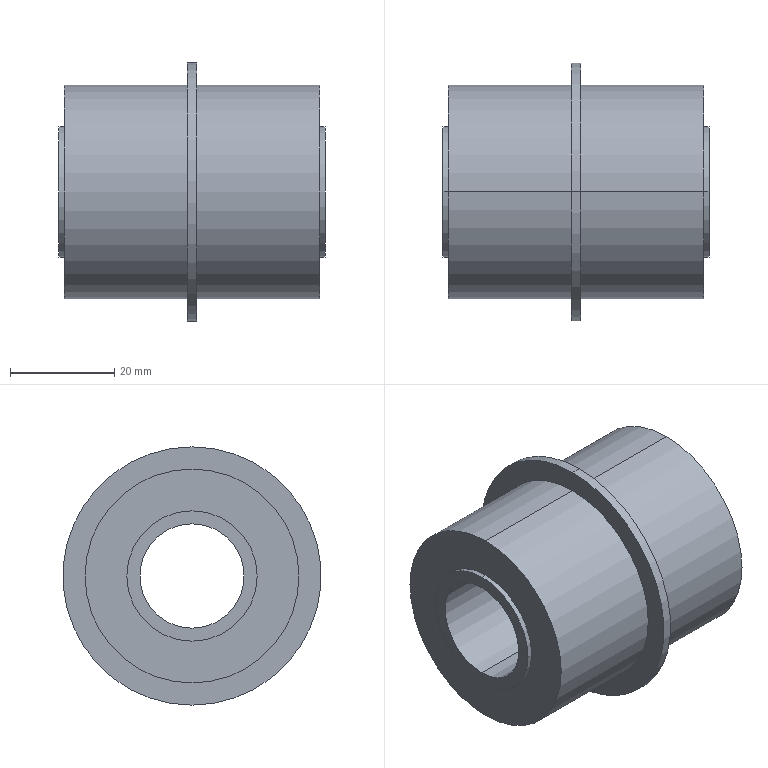Part | SolidWorks | features Revolution 1 | 1 solid | 18 faces | box 51 x 49.5 x 49.5 mm | volume 50740 mm3 | cylinder 12 | plane 6 | commonest cylinder face diameters 25 x4 41 x4 20 x2 49.5 x2
STEP:
#1=CARTESIAN_POINT('',(24.5,0.,20.5));
#2=VERTEX_POINT('',#1);
#3=CARTESIAN_POINT('',(24.5,0.,-20.5));
#4=VERTEX_POINT('',#3);
#5=CARTESIAN_POINT('',(24.5,0.,0.));
#6=DIRECTION('',(-1.,0.,0.));
#7=DIRECTION('',(0.,0.,1.));
#8=AXIS2_PLACEMENT_3D('',#5,#6,#7);
#9=CIRCLE('',#8,20.5);
#10=EDGE_CURVE('',#2,#4,#9,.T.);
#11=ORIENTED_EDGE('',*,*,#10,.T.);
#12=CARTESIAN_POINT('',(0.9,0.,-20.5));
#13=VERTEX_POINT('',#12);
#14=CARTESIAN_POINT('',(-73.222,0.,-20.5));
#15=DIRECTION('',(-1.,0.,0.));
#16=VECTOR('',#15,1000.);
#17=LINE('',#14,#16);
#18=EDGE_CURVE('',#4,#13,#17,.T.);
#19=ORIENTED_EDGE('',*,*,#18,.T.);
#20=CARTESIAN_POINT('',(0.9,0.,20.5));
#21=VERTEX_POINT('',#20);
#22=CARTESIAN_POINT('',(0.9,0.,0.));
#23=DIRECTION('',(-1.,0.,0.));
#24=DIRECTION('',(0.,0.,1.));
#25=AXIS2_PLACEMENT_3D('',#22,#23,#24);
#26=CIRCLE('',#25,20.5);
#27=EDGE_CURVE('',#21,#13,#26,.T.);
#28=ORIENTED_EDGE('',*,*,#27,.F.);
#29=CARTESIAN_POINT('',(-73.222,0.,20.5));
#30=DIRECTION('',(-1.,0.,0.));
#31=VECTOR('',#30,1000.);
#32=LINE('',#29,#31);
#33=EDGE_CURVE('',#2,#21,#32,.T.);
#34=ORIENTED_EDGE('',*,*,#33,.F.);
#35=EDGE_LOOP('',(#11,#19,#28,#34));
#36=FACE_OUTER_BOUND('',#35,.T.);
#37=CARTESIAN_POINT('',(-73.222,0.,0.));
#38=DIRECTION('',(-1.,0.,0.));
#39=DIRECTION('',(0.,0.,1.));
#40=AXIS2_PLACEMENT_3D('',#37,#38,#39);
#41=CYLINDRICAL_SURFACE('',#40,20.5);
#42=ADVANCED_FACE('',(#36),#41,.T.);
#43=CARTESIAN_POINT('',(25.5,0.,12.5));
#44=VERTEX_POINT('',#43);
#45=CARTESIAN_POINT('',(25.5,0.,-12.5));
#46=VERTEX_POINT('',#45);
#47=CARTESIAN_POINT('',(25.5,0.,0.));
#48=DIRECTION('',(-1.,0.,0.));
#49=DIRECTION('',(0.,0.,1.));
#50=AXIS2_PLACEMENT_3D('',#47,#48,#49);
#51=CIRCLE('',#50,12.5);
#52=EDGE_CURVE('',#44,#46,#51,.T.);
#53=ORIENTED_EDGE('',*,*,#52,.T.);
#54=CARTESIAN_POINT('',(24.5,0.,-12.5));
#55=VERTEX_POINT('',#54);
#56=CARTESIAN_POINT('',(-73.222,0.,-12.5));
#57=DIRECTION('',(-1.,0.,0.));
#58=VECTOR('',#57,1000.);
#59=LINE('',#56,#58);
#60=EDGE_CURVE('',#46,#55,#59,.T.);
#61=ORIENTED_EDGE('',*,*,#60,.T.);
#62=CARTESIAN_POINT('',(24.5,0.,12.5));
#63=VERTEX_POINT('',#62);
#64=CARTESIAN_POINT('',(24.5,0.,0.));
#65=DIRECTION('',(-1.,0.,0.));
#66=DIRECTION('',(0.,0.,1.));
#67=AXIS2_PLACEMENT_3D('',#64,#65,#66);
#68=CIRCLE('',#67,12.5);
#69=EDGE_CURVE('',#63,#55,#68,.T.);
#70=ORIENTED_EDGE('',*,*,#69,.F.);
#71=CARTESIAN_POINT('',(-73.222,0.,12.5));
#72=DIRECTION('',(-1.,0.,0.));
#73=VECTOR('',#72,1000.);
#74=LINE('',#71,#73);
#75=EDGE_CURVE('',#44,#63,#74,.T.);
#76=ORIENTED_EDGE('',*,*,#75,.F.);
#77=EDGE_LOOP('',(#53,#61,#70,#76));
#78=FACE_OUTER_BOUND('',#77,.T.);
#79=CARTESIAN_POINT('',(-73.222,0.,0.));
#80=DIRECTION('',(-1.,0.,0.));
#81=DIRECTION('',(0.,0.,1.));
#82=AXIS2_PLACEMENT_3D('',#79,#80,#81);
#83=CYLINDRICAL_SURFACE('',#82,12.5);
#84=ADVANCED_FACE('',(#78),#83,.T.);
#85=CARTESIAN_POINT('',(25.5,0.,-10.));
#86=VERTEX_POINT('',#85);
#87=CARTESIAN_POINT('',(25.5,0.,10.));
#88=VERTEX_POINT('',#87);
#89=CARTESIAN_POINT('',(25.5,0.,0.));
#90=DIRECTION('',(-1.,0.,0.));
#91=DIRECTION('',(0.,0.,1.));
#92=AXIS2_PLACEMENT_3D('',#89,#90,#91);
#93=CIRCLE('',#92,10.);
#94=EDGE_CURVE('',#86,#88,#93,.T.);
#95=ORIENTED_EDGE('',*,*,#94,.F.);
#96=CARTESIAN_POINT('',(-25.5,0.,-10.));
#97=VERTEX_POINT('',#96);
#98=CARTESIAN_POINT('',(-73.222,0.,-10.));
#99=DIRECTION('',(-1.,0.,0.));
#100=VECTOR('',#99,1000.);
#101=LINE('',#98,#100);
#102=EDGE_CURVE('',#86,#97,#101,.T.);
#103=ORIENTED_EDGE('',*,*,#102,.T.);
#104=CARTESIAN_POINT('',(-25.5,0.,10.));
#105=VERTEX_POINT('',#104);
#106=CARTESIAN_POINT('',(-25.5,0.,0.));
#107=DIRECTION('',(-1.,0.,0.));
#108=DIRECTION('',(0.,0.,1.));
#109=AXIS2_PLACEMENT_3D('',#106,#107,#108);
#110=CIRCLE('',#109,10.);
#111=EDGE_CURVE('',#97,#105,#110,.T.);
#112=ORIENTED_EDGE('',*,*,#111,.T.);
#113=CARTESIAN_POINT('',(-73.222,0.,10.));
#114=DIRECTION('',(-1.,0.,0.));
#115=VECTOR('',#114,1000.);
#116=LINE('',#113,#115);
#117=EDGE_CURVE('',#88,#105,#116,.T.);
#118=ORIENTED_EDGE('',*,*,#117,.F.);
#119=EDGE_LOOP('',(#95,#103,#112,#118));
#120=FACE_OUTER_BOUND('',#119,.T.);
#121=CARTESIAN_POINT('',(-73.222,0.,0.));
#122=DIRECTION('',(-1.,0.,0.));
#123=DIRECTION('',(0.,0.,1.));
#124=AXIS2_PLACEMENT_3D('',#121,#122,#123);
#125=CYLINDRICAL_SURFACE('',#124,10.);
#126=ADVANCED_FACE('',(#120),#125,.F.);
#127=CARTESIAN_POINT('',(-24.5,0.,12.5));
#128=VERTEX_POINT('',#127);
#129=CARTESIAN_POINT('',(-24.5,0.,-12.5));
#130=VERTEX_POINT('',#129);
#131=CARTESIAN_POINT('',(-24.5,0.,0.));
#132=DIRECTION('',(-1.,0.,0.));
#133=DIRECTION('',(0.,0.,1.));
#134=AXIS2_PLACEMENT_3D('',#131,#132,#133);
#135=CIRCLE('',#134,12.5);
#136=EDGE_CURVE('',#128,#130,#135,.T.);
#137=ORIENTED_EDGE('',*,*,#136,.T.);
#138=CARTESIAN_POINT('',(-25.5,0.,-12.5));
#139=VERTEX_POINT('',#138);
#140=CARTESIAN_POINT('',(-73.222,0.,-12.5));
#141=DIRECTION('',(-1.,0.,0.));
#142=VECTOR('',#141,1000.);
#143=LINE('',#140,#142);
#144=EDGE_CURVE('',#130,#139,#143,.T.);
#145=ORIENTED_EDGE('',*,*,#144,.T.);
#146=CARTESIAN_POINT('',(-25.5,0.,12.5));
#147=VERTEX_POINT('',#146);
#148=CARTESIAN_POINT('',(-25.5,0.,0.));
#149=DIRECTION('',(-1.,0.,0.));
#150=DIRECTION('',(0.,0.,1.));
#151=AXIS2_PLACEMENT_3D('',#148,#149,#150);
#152=CIRCLE('',#151,12.5);
#153=EDGE_CURVE('',#147,#139,#152,.T.);
#154=ORIENTED_EDGE('',*,*,#153,.F.);
#155=CARTESIAN_POINT('',(-73.222,0.,12.5));
#156=DIRECTION('',(-1.,0.,0.));
#157=VECTOR('',#156,1000.);
#158=LINE('',#155,#157);
#159=EDGE_CURVE('',#128,#147,#158,.T.);
#160=ORIENTED_EDGE('',*,*,#159,.F.);
#161=EDGE_LOOP('',(#137,#145,#154,#160));
#162=FACE_OUTER_BOUND('',#161,.T.);
#163=CARTESIAN_POINT('',(-73.222,0.,0.));
#164=DIRECTION('',(-1.,0.,0.));
#165=DIRECTION('',(0.,0.,1.));
#166=AXIS2_PLACEMENT_3D('',#163,#164,#165);
#167=CYLINDRICAL_SURFACE('',#166,12.5);
#168=ADVANCED_FACE('',(#162),#167,.T.);
#169=CARTESIAN_POINT('',(-0.9,0.,20.5));
#170=VERTEX_POINT('',#169);
#171=CARTESIAN_POINT('',(-0.9,0.,-20.5));
#172=VERTEX_POINT('',#171);
#173=CARTESIAN_POINT('',(-0.9,0.,0.));
#174=DIRECTION('',(-1.,0.,0.));
#175=DIRECTION('',(0.,0.,1.));
#176=AXIS2_PLACEMENT_3D('',#173,#174,#175);
#177=CIRCLE('',#176,20.5);
#178=EDGE_CURVE('',#170,#172,#177,.T.);
#179=ORIENTED_EDGE('',*,*,#178,.T.);
#180=CARTESIAN_POINT('',(-24.5,0.,-20.5));
#181=VERTEX_POINT('',#180);
#182=CARTESIAN_POINT('',(-73.222,0.,-20.5));
#183=DIRECTION('',(-1.,0.,0.));
#184=VECTOR('',#183,1000.);
#185=LINE('',#182,#184);
#186=EDGE_CURVE('',#172,#181,#185,.T.);
#187=ORIENTED_EDGE('',*,*,#186,.T.);
#188=CARTESIAN_POINT('',(-24.5,0.,20.5));
#189=VERTEX_POINT('',#188);
#190=CARTESIAN_POINT('',(-24.5,0.,0.));
#191=DIRECTION('',(-1.,0.,0.));
#192=DIRECTION('',(0.,0.,1.));
#193=AXIS2_PLACEMENT_3D('',#190,#191,#192);
#194=CIRCLE('',#193,20.5);
#195=EDGE_CURVE('',#189,#181,#194,.T.);
#196=ORIENTED_EDGE('',*,*,#195,.F.);
#197=CARTESIAN_POINT('',(-73.222,0.,20.5));
#198=DIRECTION('',(-1.,0.,0.));
#199=VECTOR('',#198,1000.);
#200=LINE('',#197,#199);
#201=EDGE_CURVE('',#170,#189,#200,.T.);
#202=ORIENTED_EDGE('',*,*,#201,.F.);
#203=EDGE_LOOP('',(#179,#187,#196,#202));
#204=FACE_OUTER_BOUND('',#203,.T.);
#205=CARTESIAN_POINT('',(-73.222,0.,0.));
#206=DIRECTION('',(-1.,0.,0.));
#207=DIRECTION('',(0.,0.,1.));
#208=AXIS2_PLACEMENT_3D('',#205,#206,#207);
#209=CYLINDRICAL_SURFACE('',#208,20.5);
#210=ADVANCED_FACE('',(#204),#209,.T.);
#211=CARTESIAN_POINT('',(0.9,0.,24.75));
#212=VERTEX_POINT('',#211);
#213=CARTESIAN_POINT('',(0.9,0.,-24.75));
#214=VERTEX_POINT('',#213);
#215=CARTESIAN_POINT('',(0.9,0.,0.));
#216=DIRECTION('',(-1.,0.,0.));
#217=DIRECTION('',(0.,0.,1.));
#218=AXIS2_PLACEMENT_3D('',#215,#216,#217);
#219=CIRCLE('',#218,24.75);
#220=EDGE_CURVE('',#212,#214,#219,.T.);
#221=ORIENTED_EDGE('',*,*,#220,.T.);
#222=CARTESIAN_POINT('',(-0.9,0.,-24.75));
#223=VERTEX_POINT('',#222);
#224=CARTESIAN_POINT('',(-73.222,0.,-24.75));
#225=DIRECTION('',(-1.,0.,0.));
#226=VECTOR('',#225,1000.);
#227=LINE('',#224,#226);
#228=EDGE_CURVE('',#214,#223,#227,.T.);
#229=ORIENTED_EDGE('',*,*,#228,.T.);
#230=CARTESIAN_POINT('',(-0.9,0.,24.75));
#231=VERTEX_POINT('',#230);
#232=CARTESIAN_POINT('',(-0.9,0.,0.));
#233=DIRECTION('',(-1.,0.,0.));
#234=DIRECTION('',(0.,0.,1.));
#235=AXIS2_PLACEMENT_3D('',#232,#233,#234);
#236=CIRCLE('',#235,24.75);
#237=EDGE_CURVE('',#231,#223,#236,.T.);
#238=ORIENTED_EDGE('',*,*,#237,.F.);
#239=CARTESIAN_POINT('',(-73.222,0.,24.75));
#240=DIRECTION('',(-1.,0.,0.));
#241=VECTOR('',#240,1000.);
#242=LINE('',#239,#241);
#243=EDGE_CURVE('',#212,#231,#242,.T.);
#244=ORIENTED_EDGE('',*,*,#243,.F.);
#245=EDGE_LOOP('',(#221,#229,#238,#244));
#246=FACE_OUTER_BOUND('',#245,.T.);
#247=CARTESIAN_POINT('',(-73.222,0.,0.));
#248=DIRECTION('',(-1.,0.,0.));
#249=DIRECTION('',(0.,0.,1.));
#250=AXIS2_PLACEMENT_3D('',#247,#248,#249);
#251=CYLINDRICAL_SURFACE('',#250,24.75);
#252=ADVANCED_FACE('',(#246),#251,.T.);
#253=ORIENTED_EDGE('',*,*,#220,.F.);
#254=CARTESIAN_POINT('',(0.9,0.,0.));
#255=DIRECTION('',(-1.,0.,0.));
#256=DIRECTION('',(0.,0.,1.));
#257=AXIS2_PLACEMENT_3D('',#254,#255,#256);
#258=CIRCLE('',#257,24.75);
#259=EDGE_CURVE('',#214,#212,#258,.T.);
#260=ORIENTED_EDGE('',*,*,#259,.F.);
#261=EDGE_LOOP('',(#253,#260));
#262=FACE_OUTER_BOUND('',#261,.T.);
#263=ORIENTED_EDGE('',*,*,#27,.T.);
#264=CARTESIAN_POINT('',(0.9,0.,0.));
#265=DIRECTION('',(-1.,0.,0.));
#266=DIRECTION('',(0.,0.,1.));
#267=AXIS2_PLACEMENT_3D('',#264,#265,#266);
#268=CIRCLE('',#267,20.5);
#269=EDGE_CURVE('',#13,#21,#268,.T.);
#270=ORIENTED_EDGE('',*,*,#269,.T.);
#271=EDGE_LOOP('',(#263,#270));
#272=FACE_BOUND('',#271,.T.);
#273=CARTESIAN_POINT('',(0.9,24.75,0.));
#274=DIRECTION('',(-1.,0.,0.));
#275=DIRECTION('',(0.,0.,1.));
#276=AXIS2_PLACEMENT_3D('',#273,#274,#275);
#277=PLANE('',#276);
#278=ADVANCED_FACE('',(#262,#272),#277,.F.);
#279=ORIENTED_EDGE('',*,*,#228,.F.);
#280=ORIENTED_EDGE('',*,*,#259,.T.);
#281=ORIENTED_EDGE('',*,*,#243,.T.);
#282=CARTESIAN_POINT('',(-0.9,0.,0.));
#283=DIRECTION('',(-1.,0.,0.));
#284=DIRECTION('',(0.,0.,1.));
#285=AXIS2_PLACEMENT_3D('',#282,#283,#284);
#286=CIRCLE('',#285,24.75);
#287=EDGE_CURVE('',#223,#231,#286,.T.);
#288=ORIENTED_EDGE('',*,*,#287,.F.);
#289=EDGE_LOOP('',(#279,#280,#281,#288));
#290=FACE_OUTER_BOUND('',#289,.T.);
#291=CARTESIAN_POINT('',(-73.222,0.,0.));
#292=DIRECTION('',(-1.,0.,0.));
#293=DIRECTION('',(0.,0.,1.));
#294=AXIS2_PLACEMENT_3D('',#291,#292,#293);
#295=CYLINDRICAL_SURFACE('',#294,24.75);
#296=ADVANCED_FACE('',(#290),#295,.T.);
#297=ORIENTED_EDGE('',*,*,#178,.F.);
#298=CARTESIAN_POINT('',(-0.9,0.,0.));
#299=DIRECTION('',(-1.,0.,0.));
#300=DIRECTION('',(0.,0.,1.));
#301=AXIS2_PLACEMENT_3D('',#298,#299,#300);
#302=CIRCLE('',#301,20.5);
#303=EDGE_CURVE('',#172,#170,#302,.T.);
#304=ORIENTED_EDGE('',*,*,#303,.F.);
#305=EDGE_LOOP('',(#297,#304));
#306=FACE_BOUND('',#305,.T.);
#307=ORIENTED_EDGE('',*,*,#237,.T.);
#308=ORIENTED_EDGE('',*,*,#287,.T.);
#309=EDGE_LOOP('',(#307,#308));
#310=FACE_OUTER_BOUND('',#309,.T.);
#311=CARTESIAN_POINT('',(-0.9,24.75,0.));
#312=DIRECTION('',(1.,0.,0.));
#313=DIRECTION('',(0.,0.,-1.));
#314=AXIS2_PLACEMENT_3D('',#311,#312,#313);
#315=PLANE('',#314);
#316=ADVANCED_FACE('',(#306,#310),#315,.F.);
#317=ORIENTED_EDGE('',*,*,#186,.F.);
#318=ORIENTED_EDGE('',*,*,#303,.T.);
#319=ORIENTED_EDGE('',*,*,#201,.T.);
#320=CARTESIAN_POINT('',(-24.5,0.,0.));
#321=DIRECTION('',(-1.,0.,0.));
#322=DIRECTION('',(0.,0.,1.));
#323=AXIS2_PLACEMENT_3D('',#320,#321,#322);
#324=CIRCLE('',#323,20.5);
#325=EDGE_CURVE('',#181,#189,#324,.T.);
#326=ORIENTED_EDGE('',*,*,#325,.F.);
#327=EDGE_LOOP('',(#317,#318,#319,#326));
#328=FACE_OUTER_BOUND('',#327,.T.);
#329=CARTESIAN_POINT('',(-73.222,0.,0.));
#330=DIRECTION('',(-1.,0.,0.));
#331=DIRECTION('',(0.,0.,1.));
#332=AXIS2_PLACEMENT_3D('',#329,#330,#331);
#333=CYLINDRICAL_SURFACE('',#332,20.5);
#334=ADVANCED_FACE('',(#328),#333,.T.);
#335=ORIENTED_EDGE('',*,*,#136,.F.);
#336=CARTESIAN_POINT('',(-24.5,0.,0.));
#337=DIRECTION('',(-1.,0.,0.));
#338=DIRECTION('',(0.,0.,1.));
#339=AXIS2_PLACEMENT_3D('',#336,#337,#338);
#340=CIRCLE('',#339,12.5);
#341=EDGE_CURVE('',#130,#128,#340,.T.);
#342=ORIENTED_EDGE('',*,*,#341,.F.);
#343=EDGE_LOOP('',(#335,#342));
#344=FACE_BOUND('',#343,.T.);
#345=ORIENTED_EDGE('',*,*,#195,.T.);
#346=ORIENTED_EDGE('',*,*,#325,.T.);
#347=EDGE_LOOP('',(#345,#346));
#348=FACE_OUTER_BOUND('',#347,.T.);
#349=CARTESIAN_POINT('',(-24.5,20.5,0.));
#350=DIRECTION('',(1.,0.,0.));
#351=DIRECTION('',(0.,0.,-1.));
#352=AXIS2_PLACEMENT_3D('',#349,#350,#351);
#353=PLANE('',#352);
#354=ADVANCED_FACE('',(#344,#348),#353,.F.);
#355=ORIENTED_EDGE('',*,*,#144,.F.);
#356=ORIENTED_EDGE('',*,*,#341,.T.);
#357=ORIENTED_EDGE('',*,*,#159,.T.);
#358=CARTESIAN_POINT('',(-25.5,0.,0.));
#359=DIRECTION('',(-1.,0.,0.));
#360=DIRECTION('',(0.,0.,1.));
#361=AXIS2_PLACEMENT_3D('',#358,#359,#360);
#362=CIRCLE('',#361,12.5);
#363=EDGE_CURVE('',#139,#147,#362,.T.);
#364=ORIENTED_EDGE('',*,*,#363,.F.);
#365=EDGE_LOOP('',(#355,#356,#357,#364));
#366=FACE_OUTER_BOUND('',#365,.T.);
#367=CARTESIAN_POINT('',(-73.222,0.,0.));
#368=DIRECTION('',(-1.,0.,0.));
#369=DIRECTION('',(0.,0.,1.));
#370=AXIS2_PLACEMENT_3D('',#367,#368,#369);
#371=CYLINDRICAL_SURFACE('',#370,12.5);
#372=ADVANCED_FACE('',(#366),#371,.T.);
#373=CARTESIAN_POINT('',(-25.5,0.,0.));
#374=DIRECTION('',(-1.,0.,0.));
#375=DIRECTION('',(0.,0.,1.));
#376=AXIS2_PLACEMENT_3D('',#373,#374,#375);
#377=CIRCLE('',#376,10.);
#378=EDGE_CURVE('',#105,#97,#377,.T.);
#379=ORIENTED_EDGE('',*,*,#378,.F.);
#380=ORIENTED_EDGE('',*,*,#111,.F.);
#381=EDGE_LOOP('',(#379,#380));
#382=FACE_BOUND('',#381,.T.);
#383=ORIENTED_EDGE('',*,*,#153,.T.);
#384=ORIENTED_EDGE('',*,*,#363,.T.);
#385=EDGE_LOOP('',(#383,#384));
#386=FACE_OUTER_BOUND('',#385,.T.);
#387=CARTESIAN_POINT('',(-25.5,12.5,0.));
#388=DIRECTION('',(1.,0.,0.));
#389=DIRECTION('',(0.,0.,-1.));
#390=AXIS2_PLACEMENT_3D('',#387,#388,#389);
#391=PLANE('',#390);
#392=ADVANCED_FACE('',(#382,#386),#391,.F.);
#393=ORIENTED_EDGE('',*,*,#102,.F.);
#394=CARTESIAN_POINT('',(25.5,0.,0.));
#395=DIRECTION('',(-1.,0.,0.));
#396=DIRECTION('',(0.,0.,1.));
#397=AXIS2_PLACEMENT_3D('',#394,#395,#396);
#398=CIRCLE('',#397,10.);
#399=EDGE_CURVE('',#88,#86,#398,.T.);
#400=ORIENTED_EDGE('',*,*,#399,.F.);
#401=ORIENTED_EDGE('',*,*,#117,.T.);
#402=ORIENTED_EDGE('',*,*,#378,.T.);
#403=EDGE_LOOP('',(#393,#400,#401,#402));
#404=FACE_OUTER_BOUND('',#403,.T.);
#405=CARTESIAN_POINT('',(-73.222,0.,0.));
#406=DIRECTION('',(-1.,0.,0.));
#407=DIRECTION('',(0.,0.,1.));
#408=AXIS2_PLACEMENT_3D('',#405,#406,#407);
#409=CYLINDRICAL_SURFACE('',#408,10.);
#410=ADVANCED_FACE('',(#404),#409,.F.);
#411=ORIENTED_EDGE('',*,*,#52,.F.);
#412=CARTESIAN_POINT('',(25.5,0.,0.));
#413=DIRECTION('',(-1.,0.,0.));
#414=DIRECTION('',(0.,0.,1.));
#415=AXIS2_PLACEMENT_3D('',#412,#413,#414);
#416=CIRCLE('',#415,12.5);
#417=EDGE_CURVE('',#46,#44,#416,.T.);
#418=ORIENTED_EDGE('',*,*,#417,.F.);
#419=EDGE_LOOP('',(#411,#418));
#420=FACE_OUTER_BOUND('',#419,.T.);
#421=ORIENTED_EDGE('',*,*,#399,.T.);
#422=ORIENTED_EDGE('',*,*,#94,.T.);
#423=EDGE_LOOP('',(#421,#422));
#424=FACE_BOUND('',#423,.T.);
#425=CARTESIAN_POINT('',(25.5,12.5,0.));
#426=DIRECTION('',(-1.,0.,0.));
#427=DIRECTION('',(0.,0.,1.));
#428=AXIS2_PLACEMENT_3D('',#425,#426,#427);
#429=PLANE('',#428);
#430=ADVANCED_FACE('',(#420,#424),#429,.F.);
#431=ORIENTED_EDGE('',*,*,#60,.F.);
#432=ORIENTED_EDGE('',*,*,#417,.T.);
#433=ORIENTED_EDGE('',*,*,#75,.T.);
#434=CARTESIAN_POINT('',(24.5,0.,0.));
#435=DIRECTION('',(-1.,0.,0.));
#436=DIRECTION('',(0.,0.,1.));
#437=AXIS2_PLACEMENT_3D('',#434,#435,#436);
#438=CIRCLE('',#437,12.5);
#439=EDGE_CURVE('',#55,#63,#438,.T.);
#440=ORIENTED_EDGE('',*,*,#439,.F.);
#441=EDGE_LOOP('',(#431,#432,#433,#440));
#442=FACE_OUTER_BOUND('',#441,.T.);
#443=CARTESIAN_POINT('',(-73.222,0.,0.));
#444=DIRECTION('',(-1.,0.,0.));
#445=DIRECTION('',(0.,0.,1.));
#446=AXIS2_PLACEMENT_3D('',#443,#444,#445);
#447=CYLINDRICAL_SURFACE('',#446,12.5);
#448=ADVANCED_FACE('',(#442),#447,.T.);
#449=ORIENTED_EDGE('',*,*,#10,.F.);
#450=CARTESIAN_POINT('',(24.5,0.,0.));
#451=DIRECTION('',(-1.,0.,0.));
#452=DIRECTION('',(0.,0.,1.));
#453=AXIS2_PLACEMENT_3D('',#450,#451,#452);
#454=CIRCLE('',#453,20.5);
#455=EDGE_CURVE('',#4,#2,#454,.T.);
#456=ORIENTED_EDGE('',*,*,#455,.F.);
#457=EDGE_LOOP('',(#449,#456));
#458=FACE_OUTER_BOUND('',#457,.T.);
#459=ORIENTED_EDGE('',*,*,#69,.T.);
#460=ORIENTED_EDGE('',*,*,#439,.T.);
#461=EDGE_LOOP('',(#459,#460));
#462=FACE_BOUND('',#461,.T.);
#463=CARTESIAN_POINT('',(24.5,20.5,0.));
#464=DIRECTION('',(-1.,0.,0.));
#465=DIRECTION('',(0.,0.,1.));
#466=AXIS2_PLACEMENT_3D('',#463,#464,#465);
#467=PLANE('',#466);
#468=ADVANCED_FACE('',(#458,#462),#467,.F.);
#469=ORIENTED_EDGE('',*,*,#18,.F.);
#470=ORIENTED_EDGE('',*,*,#455,.T.);
#471=ORIENTED_EDGE('',*,*,#33,.T.);
#472=ORIENTED_EDGE('',*,*,#269,.F.);
#473=EDGE_LOOP('',(#469,#470,#471,#472));
#474=FACE_OUTER_BOUND('',#473,.T.);
#475=CARTESIAN_POINT('',(-73.222,0.,0.));
#476=DIRECTION('',(-1.,0.,0.));
#477=DIRECTION('',(0.,0.,1.));
#478=AXIS2_PLACEMENT_3D('',#475,#476,#477);
#479=CYLINDRICAL_SURFACE('',#478,20.5);
#480=ADVANCED_FACE('',(#474),#479,.T.);
#481=CLOSED_SHELL('',(#42,#84,#126,#168,#210,#252,#278,#296,#316,#334,#354,#372,#392,#410,#430,#448,#468,#480));
#482=MANIFOLD_SOLID_BREP('',#481);
#483=CARTESIAN_POINT('',(0.,0.,0.));
#484=DIRECTION('',(0.,0.,1.));
#485=DIRECTION('',(1.,0.,0.));
#486=AXIS2_PLACEMENT_3D('',#483,#484,#485);
#487=(LENGTH_UNIT()NAMED_UNIT(*)SI_UNIT(.MILLI.,.METRE.));
#488=UNCERTAINTY_MEASURE_WITH_UNIT(LENGTH_MEASURE(0.00001),#487,'','');
#489=(NAMED_UNIT(*)PLANE_ANGLE_UNIT()SI_UNIT($,.RADIAN.));
#490=(NAMED_UNIT(*)SI_UNIT($,.STERADIAN.)SOLID_ANGLE_UNIT());
#491=(GEOMETRIC_REPRESENTATION_CONTEXT(3)GLOBAL_UNCERTAINTY_ASSIGNED_CONTEXT((#488))GLOBAL_UNIT_ASSIGNED_CONTEXT((#487,#489,#490))REPRESENTATION_CONTEXT('',''));
#492=ADVANCED_BREP_SHAPE_REPRESENTATION('',(#482,#486),#491);